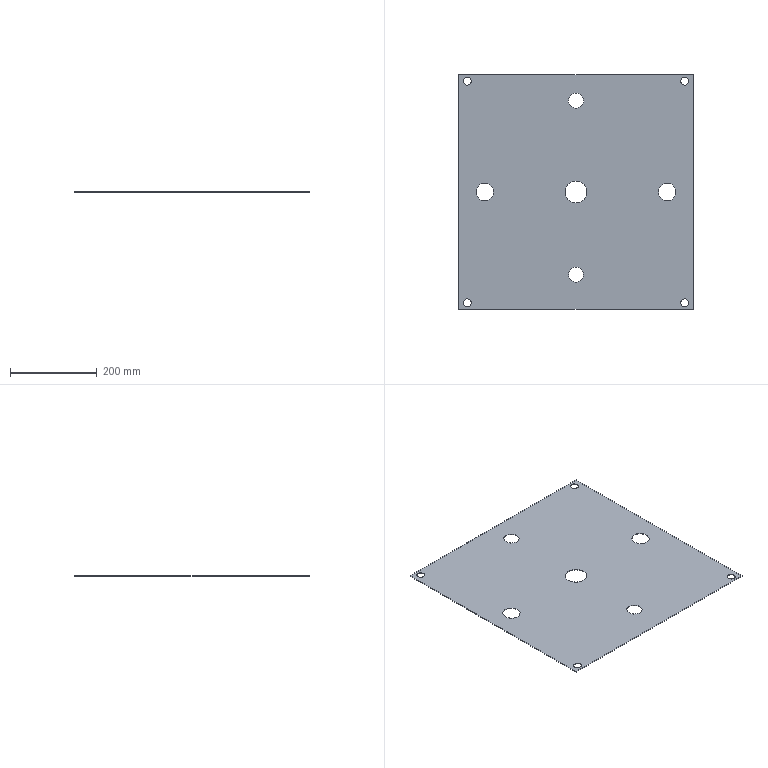Part | SolidWorks | features Cut 2, ICE 2, Extrusion 1 | 1 solid | 24 faces | box 540 x 540 x 1 mm | volume 284181 mm3 | cylinder 18 | plane 6 | commonest cylinder face diameters 18 x8 35 x4 40 x4 50 x2
STEP:
#1=CARTESIAN_POINT('',(17.5,210.,1.));
#2=VERTEX_POINT('',#1);
#3=CARTESIAN_POINT('',(-17.5,210.,1.));
#4=VERTEX_POINT('',#3);
#5=CARTESIAN_POINT('',(0.,210.,1.));
#6=DIRECTION('',(0.,0.,-1.));
#7=DIRECTION('',(-1.,0.,0.));
#8=AXIS2_PLACEMENT_3D('',#5,#6,#7);
#9=CIRCLE('',#8,17.5);
#10=EDGE_CURVE('',#2,#4,#9,.T.);
#11=ORIENTED_EDGE('',*,*,#10,.F.);
#12=CARTESIAN_POINT('',(17.5,210.,0.));
#13=VERTEX_POINT('',#12);
#14=CARTESIAN_POINT('',(17.5,210.,1.));
#15=DIRECTION('',(0.,0.,-1.));
#16=VECTOR('',#15,1000.);
#17=LINE('',#14,#16);
#18=EDGE_CURVE('',#2,#13,#17,.T.);
#19=ORIENTED_EDGE('',*,*,#18,.T.);
#20=CARTESIAN_POINT('',(-17.5,210.,0.));
#21=VERTEX_POINT('',#20);
#22=CARTESIAN_POINT('',(0.,210.,0.));
#23=DIRECTION('',(0.,0.,-1.));
#24=DIRECTION('',(-1.,0.,0.));
#25=AXIS2_PLACEMENT_3D('',#22,#23,#24);
#26=CIRCLE('',#25,17.5);
#27=EDGE_CURVE('',#13,#21,#26,.T.);
#28=ORIENTED_EDGE('',*,*,#27,.T.);
#29=CARTESIAN_POINT('',(-17.5,210.,1.));
#30=DIRECTION('',(0.,0.,-1.));
#31=VECTOR('',#30,1000.);
#32=LINE('',#29,#31);
#33=EDGE_CURVE('',#4,#21,#32,.T.);
#34=ORIENTED_EDGE('',*,*,#33,.F.);
#35=EDGE_LOOP('',(#11,#19,#28,#34));
#36=FACE_OUTER_BOUND('',#35,.T.);
#37=CARTESIAN_POINT('',(0.,210.,1.));
#38=DIRECTION('',(0.,0.,-1.));
#39=DIRECTION('',(-1.,0.,0.));
#40=AXIS2_PLACEMENT_3D('',#37,#38,#39);
#41=CYLINDRICAL_SURFACE('',#40,17.5);
#42=ADVANCED_FACE('',(#36),#41,.F.);
#43=CARTESIAN_POINT('',(17.5,-190.,1.));
#44=VERTEX_POINT('',#43);
#45=CARTESIAN_POINT('',(-17.5,-190.,1.));
#46=VERTEX_POINT('',#45);
#47=CARTESIAN_POINT('',(0.,-190.,1.));
#48=DIRECTION('',(0.,0.,-1.));
#49=DIRECTION('',(-1.,0.,0.));
#50=AXIS2_PLACEMENT_3D('',#47,#48,#49);
#51=CIRCLE('',#50,17.5);
#52=EDGE_CURVE('',#44,#46,#51,.T.);
#53=ORIENTED_EDGE('',*,*,#52,.F.);
#54=CARTESIAN_POINT('',(17.5,-190.,0.));
#55=VERTEX_POINT('',#54);
#56=CARTESIAN_POINT('',(17.5,-190.,1.));
#57=DIRECTION('',(0.,0.,-1.));
#58=VECTOR('',#57,1000.);
#59=LINE('',#56,#58);
#60=EDGE_CURVE('',#44,#55,#59,.T.);
#61=ORIENTED_EDGE('',*,*,#60,.T.);
#62=CARTESIAN_POINT('',(-17.5,-190.,0.));
#63=VERTEX_POINT('',#62);
#64=CARTESIAN_POINT('',(0.,-190.,0.));
#65=DIRECTION('',(0.,0.,-1.));
#66=DIRECTION('',(-1.,0.,0.));
#67=AXIS2_PLACEMENT_3D('',#64,#65,#66);
#68=CIRCLE('',#67,17.5);
#69=EDGE_CURVE('',#55,#63,#68,.T.);
#70=ORIENTED_EDGE('',*,*,#69,.T.);
#71=CARTESIAN_POINT('',(-17.5,-190.,1.));
#72=DIRECTION('',(0.,0.,-1.));
#73=VECTOR('',#72,1000.);
#74=LINE('',#71,#73);
#75=EDGE_CURVE('',#46,#63,#74,.T.);
#76=ORIENTED_EDGE('',*,*,#75,.F.);
#77=EDGE_LOOP('',(#53,#61,#70,#76));
#78=FACE_OUTER_BOUND('',#77,.T.);
#79=CARTESIAN_POINT('',(0.,-190.,1.));
#80=DIRECTION('',(0.,0.,-1.));
#81=DIRECTION('',(-1.,0.,0.));
#82=AXIS2_PLACEMENT_3D('',#79,#80,#81);
#83=CYLINDRICAL_SURFACE('',#82,17.5);
#84=ADVANCED_FACE('',(#78),#83,.F.);
#85=CARTESIAN_POINT('',(-25.,0.,0.));
#86=VERTEX_POINT('',#85);
#87=CARTESIAN_POINT('',(25.,0.,0.));
#88=VERTEX_POINT('',#87);
#89=CARTESIAN_POINT('',(0.,0.,0.));
#90=DIRECTION('',(0.,0.,1.));
#91=DIRECTION('',(1.,0.,0.));
#92=AXIS2_PLACEMENT_3D('',#89,#90,#91);
#93=CIRCLE('',#92,25.);
#94=EDGE_CURVE('',#86,#88,#93,.T.);
#95=ORIENTED_EDGE('',*,*,#94,.F.);
#96=CARTESIAN_POINT('',(-25.,0.,1.));
#97=VERTEX_POINT('',#96);
#98=CARTESIAN_POINT('',(-25.,0.,-9.));
#99=DIRECTION('',(0.,0.,1.));
#100=VECTOR('',#99,1000.);
#101=LINE('',#98,#100);
#102=EDGE_CURVE('',#86,#97,#101,.T.);
#103=ORIENTED_EDGE('',*,*,#102,.T.);
#104=CARTESIAN_POINT('',(25.,0.,1.));
#105=VERTEX_POINT('',#104);
#106=CARTESIAN_POINT('',(0.,0.,1.));
#107=DIRECTION('',(0.,0.,1.));
#108=DIRECTION('',(1.,0.,0.));
#109=AXIS2_PLACEMENT_3D('',#106,#107,#108);
#110=CIRCLE('',#109,25.);
#111=EDGE_CURVE('',#97,#105,#110,.T.);
#112=ORIENTED_EDGE('',*,*,#111,.T.);
#113=CARTESIAN_POINT('',(25.,0.,-9.));
#114=DIRECTION('',(0.,0.,1.));
#115=VECTOR('',#114,1000.);
#116=LINE('',#113,#115);
#117=EDGE_CURVE('',#88,#105,#116,.T.);
#118=ORIENTED_EDGE('',*,*,#117,.F.);
#119=EDGE_LOOP('',(#95,#103,#112,#118));
#120=FACE_OUTER_BOUND('',#119,.T.);
#121=CARTESIAN_POINT('',(0.,0.,-9.));
#122=DIRECTION('',(0.,0.,1.));
#123=DIRECTION('',(1.,0.,0.));
#124=AXIS2_PLACEMENT_3D('',#121,#122,#123);
#125=CYLINDRICAL_SURFACE('',#124,25.);
#126=ADVANCED_FACE('',(#120),#125,.F.);
#127=CARTESIAN_POINT('',(190.,0.,0.));
#128=VERTEX_POINT('',#127);
#129=CARTESIAN_POINT('',(230.,0.,0.));
#130=VERTEX_POINT('',#129);
#131=CARTESIAN_POINT('',(210.,0.,0.));
#132=DIRECTION('',(0.,0.,1.));
#133=DIRECTION('',(1.,0.,0.));
#134=AXIS2_PLACEMENT_3D('',#131,#132,#133);
#135=CIRCLE('',#134,20.);
#136=EDGE_CURVE('',#128,#130,#135,.T.);
#137=ORIENTED_EDGE('',*,*,#136,.F.);
#138=CARTESIAN_POINT('',(190.,0.,1.));
#139=VERTEX_POINT('',#138);
#140=CARTESIAN_POINT('',(190.,0.,0.));
#141=DIRECTION('',(0.,0.,1.));
#142=VECTOR('',#141,1000.);
#143=LINE('',#140,#142);
#144=EDGE_CURVE('',#128,#139,#143,.T.);
#145=ORIENTED_EDGE('',*,*,#144,.T.);
#146=CARTESIAN_POINT('',(230.,0.,1.));
#147=VERTEX_POINT('',#146);
#148=CARTESIAN_POINT('',(210.,0.,1.));
#149=DIRECTION('',(0.,0.,1.));
#150=DIRECTION('',(1.,0.,0.));
#151=AXIS2_PLACEMENT_3D('',#148,#149,#150);
#152=CIRCLE('',#151,20.);
#153=EDGE_CURVE('',#139,#147,#152,.T.);
#154=ORIENTED_EDGE('',*,*,#153,.T.);
#155=CARTESIAN_POINT('',(230.,0.,0.));
#156=DIRECTION('',(0.,0.,1.));
#157=VECTOR('',#156,1000.);
#158=LINE('',#155,#157);
#159=EDGE_CURVE('',#130,#147,#158,.T.);
#160=ORIENTED_EDGE('',*,*,#159,.F.);
#161=EDGE_LOOP('',(#137,#145,#154,#160));
#162=FACE_OUTER_BOUND('',#161,.T.);
#163=CARTESIAN_POINT('',(210.,0.,0.));
#164=DIRECTION('',(0.,0.,1.));
#165=DIRECTION('',(1.,0.,0.));
#166=AXIS2_PLACEMENT_3D('',#163,#164,#165);
#167=CYLINDRICAL_SURFACE('',#166,20.);
#168=ADVANCED_FACE('',(#162),#167,.F.);
#169=CARTESIAN_POINT('',(-230.,0.,0.));
#170=VERTEX_POINT('',#169);
#171=CARTESIAN_POINT('',(-190.,0.,0.));
#172=VERTEX_POINT('',#171);
#173=CARTESIAN_POINT('',(-210.,0.,0.));
#174=DIRECTION('',(0.,0.,1.));
#175=DIRECTION('',(1.,0.,0.));
#176=AXIS2_PLACEMENT_3D('',#173,#174,#175);
#177=CIRCLE('',#176,20.);
#178=EDGE_CURVE('',#170,#172,#177,.T.);
#179=ORIENTED_EDGE('',*,*,#178,.F.);
#180=CARTESIAN_POINT('',(-230.,0.,1.));
#181=VERTEX_POINT('',#180);
#182=CARTESIAN_POINT('',(-230.,0.,0.));
#183=DIRECTION('',(0.,0.,1.));
#184=VECTOR('',#183,1000.);
#185=LINE('',#182,#184);
#186=EDGE_CURVE('',#170,#181,#185,.T.);
#187=ORIENTED_EDGE('',*,*,#186,.T.);
#188=CARTESIAN_POINT('',(-190.,0.,1.));
#189=VERTEX_POINT('',#188);
#190=CARTESIAN_POINT('',(-210.,0.,1.));
#191=DIRECTION('',(0.,0.,1.));
#192=DIRECTION('',(1.,0.,0.));
#193=AXIS2_PLACEMENT_3D('',#190,#191,#192);
#194=CIRCLE('',#193,20.);
#195=EDGE_CURVE('',#181,#189,#194,.T.);
#196=ORIENTED_EDGE('',*,*,#195,.T.);
#197=CARTESIAN_POINT('',(-190.,0.,0.));
#198=DIRECTION('',(0.,0.,1.));
#199=VECTOR('',#198,1000.);
#200=LINE('',#197,#199);
#201=EDGE_CURVE('',#172,#189,#200,.T.);
#202=ORIENTED_EDGE('',*,*,#201,.F.);
#203=EDGE_LOOP('',(#179,#187,#196,#202));
#204=FACE_OUTER_BOUND('',#203,.T.);
#205=CARTESIAN_POINT('',(-210.,0.,0.));
#206=DIRECTION('',(0.,0.,1.));
#207=DIRECTION('',(1.,0.,0.));
#208=AXIS2_PLACEMENT_3D('',#205,#206,#207);
#209=CYLINDRICAL_SURFACE('',#208,20.);
#210=ADVANCED_FACE('',(#204),#209,.F.);
#211=CARTESIAN_POINT('',(259.,255.,1.));
#212=VERTEX_POINT('',#211);
#213=CARTESIAN_POINT('',(241.,255.,1.));
#214=VERTEX_POINT('',#213);
#215=CARTESIAN_POINT('',(250.,255.,1.));
#216=DIRECTION('',(0.,0.,-1.));
#217=DIRECTION('',(-1.,0.,0.));
#218=AXIS2_PLACEMENT_3D('',#215,#216,#217);
#219=CIRCLE('',#218,9.);
#220=EDGE_CURVE('',#212,#214,#219,.T.);
#221=ORIENTED_EDGE('',*,*,#220,.F.);
#222=CARTESIAN_POINT('',(259.,255.,0.));
#223=VERTEX_POINT('',#222);
#224=CARTESIAN_POINT('',(259.,255.,1.));
#225=DIRECTION('',(0.,0.,-1.));
#226=VECTOR('',#225,1000.);
#227=LINE('',#224,#226);
#228=EDGE_CURVE('',#212,#223,#227,.T.);
#229=ORIENTED_EDGE('',*,*,#228,.T.);
#230=CARTESIAN_POINT('',(241.,255.,0.));
#231=VERTEX_POINT('',#230);
#232=CARTESIAN_POINT('',(250.,255.,0.));
#233=DIRECTION('',(0.,0.,-1.));
#234=DIRECTION('',(-1.,0.,0.));
#235=AXIS2_PLACEMENT_3D('',#232,#233,#234);
#236=CIRCLE('',#235,9.);
#237=EDGE_CURVE('',#223,#231,#236,.T.);
#238=ORIENTED_EDGE('',*,*,#237,.T.);
#239=CARTESIAN_POINT('',(241.,255.,1.));
#240=DIRECTION('',(0.,0.,-1.));
#241=VECTOR('',#240,1000.);
#242=LINE('',#239,#241);
#243=EDGE_CURVE('',#214,#231,#242,.T.);
#244=ORIENTED_EDGE('',*,*,#243,.F.);
#245=EDGE_LOOP('',(#221,#229,#238,#244));
#246=FACE_OUTER_BOUND('',#245,.T.);
#247=CARTESIAN_POINT('',(250.,255.,1.));
#248=DIRECTION('',(0.,0.,-1.));
#249=DIRECTION('',(-1.,0.,0.));
#250=AXIS2_PLACEMENT_3D('',#247,#248,#249);
#251=CYLINDRICAL_SURFACE('',#250,9.);
#252=ADVANCED_FACE('',(#246),#251,.F.);
#253=CARTESIAN_POINT('',(-241.,255.,1.));
#254=VERTEX_POINT('',#253);
#255=CARTESIAN_POINT('',(-259.,255.,1.));
#256=VERTEX_POINT('',#255);
#257=CARTESIAN_POINT('',(-250.,255.,1.));
#258=DIRECTION('',(0.,0.,-1.));
#259=DIRECTION('',(-1.,0.,0.));
#260=AXIS2_PLACEMENT_3D('',#257,#258,#259);
#261=CIRCLE('',#260,9.);
#262=EDGE_CURVE('',#254,#256,#261,.T.);
#263=ORIENTED_EDGE('',*,*,#262,.F.);
#264=CARTESIAN_POINT('',(-241.,255.,0.));
#265=VERTEX_POINT('',#264);
#266=CARTESIAN_POINT('',(-241.,255.,1.));
#267=DIRECTION('',(0.,0.,-1.));
#268=VECTOR('',#267,1000.);
#269=LINE('',#266,#268);
#270=EDGE_CURVE('',#254,#265,#269,.T.);
#271=ORIENTED_EDGE('',*,*,#270,.T.);
#272=CARTESIAN_POINT('',(-259.,255.,0.));
#273=VERTEX_POINT('',#272);
#274=CARTESIAN_POINT('',(-250.,255.,0.));
#275=DIRECTION('',(0.,0.,-1.));
#276=DIRECTION('',(-1.,0.,0.));
#277=AXIS2_PLACEMENT_3D('',#274,#275,#276);
#278=CIRCLE('',#277,9.);
#279=EDGE_CURVE('',#265,#273,#278,.T.);
#280=ORIENTED_EDGE('',*,*,#279,.T.);
#281=CARTESIAN_POINT('',(-259.,255.,1.));
#282=DIRECTION('',(0.,0.,-1.));
#283=VECTOR('',#282,1000.);
#284=LINE('',#281,#283);
#285=EDGE_CURVE('',#256,#273,#284,.T.);
#286=ORIENTED_EDGE('',*,*,#285,.F.);
#287=EDGE_LOOP('',(#263,#271,#280,#286));
#288=FACE_OUTER_BOUND('',#287,.T.);
#289=CARTESIAN_POINT('',(-250.,255.,1.));
#290=DIRECTION('',(0.,0.,-1.));
#291=DIRECTION('',(-1.,0.,0.));
#292=AXIS2_PLACEMENT_3D('',#289,#290,#291);
#293=CYLINDRICAL_SURFACE('',#292,9.);
#294=ADVANCED_FACE('',(#288),#293,.F.);
#295=CARTESIAN_POINT('',(259.,-255.,1.));
#296=VERTEX_POINT('',#295);
#297=CARTESIAN_POINT('',(241.,-255.,1.));
#298=VERTEX_POINT('',#297);
#299=CARTESIAN_POINT('',(250.,-255.,1.));
#300=DIRECTION('',(0.,0.,-1.));
#301=DIRECTION('',(-1.,0.,0.));
#302=AXIS2_PLACEMENT_3D('',#299,#300,#301);
#303=CIRCLE('',#302,9.);
#304=EDGE_CURVE('',#296,#298,#303,.T.);
#305=ORIENTED_EDGE('',*,*,#304,.F.);
#306=CARTESIAN_POINT('',(259.,-255.,0.));
#307=VERTEX_POINT('',#306);
#308=CARTESIAN_POINT('',(259.,-255.,1.));
#309=DIRECTION('',(0.,0.,-1.));
#310=VECTOR('',#309,1000.);
#311=LINE('',#308,#310);
#312=EDGE_CURVE('',#296,#307,#311,.T.);
#313=ORIENTED_EDGE('',*,*,#312,.T.);
#314=CARTESIAN_POINT('',(241.,-255.,0.));
#315=VERTEX_POINT('',#314);
#316=CARTESIAN_POINT('',(250.,-255.,0.));
#317=DIRECTION('',(0.,0.,-1.));
#318=DIRECTION('',(-1.,0.,0.));
#319=AXIS2_PLACEMENT_3D('',#316,#317,#318);
#320=CIRCLE('',#319,9.);
#321=EDGE_CURVE('',#307,#315,#320,.T.);
#322=ORIENTED_EDGE('',*,*,#321,.T.);
#323=CARTESIAN_POINT('',(241.,-255.,1.));
#324=DIRECTION('',(0.,0.,-1.));
#325=VECTOR('',#324,1000.);
#326=LINE('',#323,#325);
#327=EDGE_CURVE('',#298,#315,#326,.T.);
#328=ORIENTED_EDGE('',*,*,#327,.F.);
#329=EDGE_LOOP('',(#305,#313,#322,#328));
#330=FACE_OUTER_BOUND('',#329,.T.);
#331=CARTESIAN_POINT('',(250.,-255.,1.));
#332=DIRECTION('',(0.,0.,-1.));
#333=DIRECTION('',(-1.,0.,0.));
#334=AXIS2_PLACEMENT_3D('',#331,#332,#333);
#335=CYLINDRICAL_SURFACE('',#334,9.);
#336=ADVANCED_FACE('',(#330),#335,.F.);
#337=CARTESIAN_POINT('',(-241.,-255.,1.));
#338=VERTEX_POINT('',#337);
#339=CARTESIAN_POINT('',(-259.,-255.,1.));
#340=VERTEX_POINT('',#339);
#341=CARTESIAN_POINT('',(-250.,-255.,1.));
#342=DIRECTION('',(0.,0.,-1.));
#343=DIRECTION('',(-1.,0.,0.));
#344=AXIS2_PLACEMENT_3D('',#341,#342,#343);
#345=CIRCLE('',#344,9.);
#346=EDGE_CURVE('',#338,#340,#345,.T.);
#347=ORIENTED_EDGE('',*,*,#346,.F.);
#348=CARTESIAN_POINT('',(-241.,-255.,0.));
#349=VERTEX_POINT('',#348);
#350=CARTESIAN_POINT('',(-241.,-255.,1.));
#351=DIRECTION('',(0.,0.,-1.));
#352=VECTOR('',#351,1000.);
#353=LINE('',#350,#352);
#354=EDGE_CURVE('',#338,#349,#353,.T.);
#355=ORIENTED_EDGE('',*,*,#354,.T.);
#356=CARTESIAN_POINT('',(-259.,-255.,0.));
#357=VERTEX_POINT('',#356);
#358=CARTESIAN_POINT('',(-250.,-255.,0.));
#359=DIRECTION('',(0.,0.,-1.));
#360=DIRECTION('',(-1.,0.,0.));
#361=AXIS2_PLACEMENT_3D('',#358,#359,#360);
#362=CIRCLE('',#361,9.);
#363=EDGE_CURVE('',#349,#357,#362,.T.);
#364=ORIENTED_EDGE('',*,*,#363,.T.);
#365=CARTESIAN_POINT('',(-259.,-255.,1.));
#366=DIRECTION('',(0.,0.,-1.));
#367=VECTOR('',#366,1000.);
#368=LINE('',#365,#367);
#369=EDGE_CURVE('',#340,#357,#368,.T.);
#370=ORIENTED_EDGE('',*,*,#369,.F.);
#371=EDGE_LOOP('',(#347,#355,#364,#370));
#372=FACE_OUTER_BOUND('',#371,.T.);
#373=CARTESIAN_POINT('',(-250.,-255.,1.));
#374=DIRECTION('',(0.,0.,-1.));
#375=DIRECTION('',(-1.,0.,0.));
#376=AXIS2_PLACEMENT_3D('',#373,#374,#375);
#377=CYLINDRICAL_SURFACE('',#376,9.);
#378=ADVANCED_FACE('',(#372),#377,.F.);
#379=CARTESIAN_POINT('',(270.,-270.,0.));
#380=VERTEX_POINT('',#379);
#381=CARTESIAN_POINT('',(270.,270.,0.));
#382=VERTEX_POINT('',#381);
#383=CARTESIAN_POINT('',(270.,270.,0.));
#384=DIRECTION('',(0.,1.,0.));
#385=VECTOR('',#384,1000.);
#386=LINE('',#383,#385);
#387=EDGE_CURVE('',#380,#382,#386,.T.);
#388=ORIENTED_EDGE('',*,*,#387,.T.);
#389=CARTESIAN_POINT('',(270.,270.,1.));
#390=VERTEX_POINT('',#389);
#391=CARTESIAN_POINT('',(270.,270.,1.));
#392=DIRECTION('',(0.,0.,-1.));
#393=VECTOR('',#392,1000.);
#394=LINE('',#391,#393);
#395=EDGE_CURVE('',#390,#382,#394,.T.);
#396=ORIENTED_EDGE('',*,*,#395,.F.);
#397=CARTESIAN_POINT('',(270.,-270.,1.));
#398=VERTEX_POINT('',#397);
#399=CARTESIAN_POINT('',(270.,270.,1.));
#400=DIRECTION('',(0.,1.,0.));
#401=VECTOR('',#400,1000.);
#402=LINE('',#399,#401);
#403=EDGE_CURVE('',#398,#390,#402,.T.);
#404=ORIENTED_EDGE('',*,*,#403,.F.);
#405=CARTESIAN_POINT('',(270.,-270.,1.));
#406=DIRECTION('',(0.,0.,-1.));
#407=VECTOR('',#406,1000.);
#408=LINE('',#405,#407);
#409=EDGE_CURVE('',#398,#380,#408,.T.);
#410=ORIENTED_EDGE('',*,*,#409,.T.);
#411=EDGE_LOOP('',(#388,#396,#404,#410));
#412=FACE_OUTER_BOUND('',#411,.T.);
#413=CARTESIAN_POINT('',(270.,270.,1.));
#414=DIRECTION('',(-1.,0.,0.));
#415=DIRECTION('',(0.,-1.,0.));
#416=AXIS2_PLACEMENT_3D('',#413,#414,#415);
#417=PLANE('',#416);
#418=ADVANCED_FACE('',(#412),#417,.F.);
#419=CARTESIAN_POINT('',(-270.,270.,0.));
#420=VERTEX_POINT('',#419);
#421=CARTESIAN_POINT('',(-270.,270.,0.));
#422=DIRECTION('',(-1.,0.,0.));
#423=VECTOR('',#422,1000.);
#424=LINE('',#421,#423);
#425=EDGE_CURVE('',#382,#420,#424,.T.);
#426=ORIENTED_EDGE('',*,*,#425,.T.);
#427=CARTESIAN_POINT('',(-270.,270.,1.));
#428=VERTEX_POINT('',#427);
#429=CARTESIAN_POINT('',(-270.,270.,1.));
#430=DIRECTION('',(0.,0.,-1.));
#431=VECTOR('',#430,1000.);
#432=LINE('',#429,#431);
#433=EDGE_CURVE('',#428,#420,#432,.T.);
#434=ORIENTED_EDGE('',*,*,#433,.F.);
#435=CARTESIAN_POINT('',(-270.,270.,1.));
#436=DIRECTION('',(-1.,0.,0.));
#437=VECTOR('',#436,1000.);
#438=LINE('',#435,#437);
#439=EDGE_CURVE('',#390,#428,#438,.T.);
#440=ORIENTED_EDGE('',*,*,#439,.F.);
#441=ORIENTED_EDGE('',*,*,#395,.T.);
#442=EDGE_LOOP('',(#426,#434,#440,#441));
#443=FACE_OUTER_BOUND('',#442,.T.);
#444=CARTESIAN_POINT('',(-270.,270.,1.));
#445=DIRECTION('',(0.,-1.,0.));
#446=DIRECTION('',(0.,0.,-1.));
#447=AXIS2_PLACEMENT_3D('',#444,#445,#446);
#448=PLANE('',#447);
#449=ADVANCED_FACE('',(#443),#448,.F.);
#450=CARTESIAN_POINT('',(-270.,-270.,0.));
#451=VERTEX_POINT('',#450);
#452=CARTESIAN_POINT('',(-270.,270.,0.));
#453=DIRECTION('',(0.,-1.,0.));
#454=VECTOR('',#453,1000.);
#455=LINE('',#452,#454);
#456=EDGE_CURVE('',#420,#451,#455,.T.);
#457=ORIENTED_EDGE('',*,*,#456,.T.);
#458=CARTESIAN_POINT('',(-270.,-270.,1.));
#459=VERTEX_POINT('',#458);
#460=CARTESIAN_POINT('',(-270.,-270.,1.));
#461=DIRECTION('',(0.,0.,-1.));
#462=VECTOR('',#461,1000.);
#463=LINE('',#460,#462);
#464=EDGE_CURVE('',#459,#451,#463,.T.);
#465=ORIENTED_EDGE('',*,*,#464,.F.);
#466=CARTESIAN_POINT('',(-270.,270.,1.));
#467=DIRECTION('',(0.,-1.,0.));
#468=VECTOR('',#467,1000.);
#469=LINE('',#466,#468);
#470=EDGE_CURVE('',#428,#459,#469,.T.);
#471=ORIENTED_EDGE('',*,*,#470,.F.);
#472=ORIENTED_EDGE('',*,*,#433,.T.);
#473=EDGE_LOOP('',(#457,#465,#471,#472));
#474=FACE_OUTER_BOUND('',#473,.T.);
#475=CARTESIAN_POINT('',(-270.,270.,1.));
#476=DIRECTION('',(1.,0.,0.));
#477=DIRECTION('',(0.,1.,0.));
#478=AXIS2_PLACEMENT_3D('',#475,#476,#477);
#479=PLANE('',#478);
#480=ADVANCED_FACE('',(#474),#479,.F.);
#481=CARTESIAN_POINT('',(-270.,-270.,0.));
#482=DIRECTION('',(1.,0.,0.));
#483=VECTOR('',#482,1000.);
#484=LINE('',#481,#483);
#485=EDGE_CURVE('',#451,#380,#484,.T.);
#486=ORIENTED_EDGE('',*,*,#485,.T.);
#487=ORIENTED_EDGE('',*,*,#409,.F.);
#488=CARTESIAN_POINT('',(-270.,-270.,1.));
#489=DIRECTION('',(1.,0.,0.));
#490=VECTOR('',#489,1000.);
#491=LINE('',#488,#490);
#492=EDGE_CURVE('',#459,#398,#491,.T.);
#493=ORIENTED_EDGE('',*,*,#492,.F.);
#494=ORIENTED_EDGE('',*,*,#464,.T.);
#495=EDGE_LOOP('',(#486,#487,#493,#494));
#496=FACE_OUTER_BOUND('',#495,.T.);
#497=CARTESIAN_POINT('',(-270.,-270.,1.));
#498=DIRECTION('',(0.,1.,0.));
#499=DIRECTION('',(0.,0.,1.));
#500=AXIS2_PLACEMENT_3D('',#497,#498,#499);
#501=PLANE('',#500);
#502=ADVANCED_FACE('',(#496),#501,.F.);
#503=CARTESIAN_POINT('',(0.,210.,1.));
#504=DIRECTION('',(0.,0.,-1.));
#505=DIRECTION('',(-1.,0.,0.));
#506=AXIS2_PLACEMENT_3D('',#503,#504,#505);
#507=CIRCLE('',#506,17.5);
#508=EDGE_CURVE('',#4,#2,#507,.T.);
#509=ORIENTED_EDGE('',*,*,#508,.T.);
#510=ORIENTED_EDGE('',*,*,#10,.T.);
#511=EDGE_LOOP('',(#509,#510));
#512=FACE_BOUND('',#511,.T.);
#513=CARTESIAN_POINT('',(0.,-190.,1.));
#514=DIRECTION('',(0.,0.,-1.));
#515=DIRECTION('',(-1.,0.,0.));
#516=AXIS2_PLACEMENT_3D('',#513,#514,#515);
#517=CIRCLE('',#516,17.5);
#518=EDGE_CURVE('',#46,#44,#517,.T.);
#519=ORIENTED_EDGE('',*,*,#518,.T.);
#520=ORIENTED_EDGE('',*,*,#52,.T.);
#521=EDGE_LOOP('',(#519,#520));
#522=FACE_BOUND('',#521,.T.);
#523=CARTESIAN_POINT('',(0.,0.,1.));
#524=DIRECTION('',(0.,0.,1.));
#525=DIRECTION('',(1.,0.,0.));
#526=AXIS2_PLACEMENT_3D('',#523,#524,#525);
#527=CIRCLE('',#526,25.);
#528=EDGE_CURVE('',#105,#97,#527,.T.);
#529=ORIENTED_EDGE('',*,*,#528,.F.);
#530=ORIENTED_EDGE('',*,*,#111,.F.);
#531=EDGE_LOOP('',(#529,#530));
#532=FACE_BOUND('',#531,.T.);
#533=CARTESIAN_POINT('',(210.,0.,1.));
#534=DIRECTION('',(0.,0.,1.));
#535=DIRECTION('',(1.,0.,0.));
#536=AXIS2_PLACEMENT_3D('',#533,#534,#535);
#537=CIRCLE('',#536,20.);
#538=EDGE_CURVE('',#147,#139,#537,.T.);
#539=ORIENTED_EDGE('',*,*,#538,.F.);
#540=ORIENTED_EDGE('',*,*,#153,.F.);
#541=EDGE_LOOP('',(#539,#540));
#542=FACE_BOUND('',#541,.T.);
#543=CARTESIAN_POINT('',(-210.,0.,1.));
#544=DIRECTION('',(0.,0.,1.));
#545=DIRECTION('',(1.,0.,0.));
#546=AXIS2_PLACEMENT_3D('',#543,#544,#545);
#547=CIRCLE('',#546,20.);
#548=EDGE_CURVE('',#189,#181,#547,.T.);
#549=ORIENTED_EDGE('',*,*,#548,.F.);
#550=ORIENTED_EDGE('',*,*,#195,.F.);
#551=EDGE_LOOP('',(#549,#550));
#552=FACE_BOUND('',#551,.T.);
#553=CARTESIAN_POINT('',(250.,255.,1.));
#554=DIRECTION('',(0.,0.,-1.));
#555=DIRECTION('',(-1.,0.,0.));
#556=AXIS2_PLACEMENT_3D('',#553,#554,#555);
#557=CIRCLE('',#556,9.);
#558=EDGE_CURVE('',#214,#212,#557,.T.);
#559=ORIENTED_EDGE('',*,*,#558,.T.);
#560=ORIENTED_EDGE('',*,*,#220,.T.);
#561=EDGE_LOOP('',(#559,#560));
#562=FACE_BOUND('',#561,.T.);
#563=CARTESIAN_POINT('',(-250.,255.,1.));
#564=DIRECTION('',(0.,0.,-1.));
#565=DIRECTION('',(-1.,0.,0.));
#566=AXIS2_PLACEMENT_3D('',#563,#564,#565);
#567=CIRCLE('',#566,9.);
#568=EDGE_CURVE('',#256,#254,#567,.T.);
#569=ORIENTED_EDGE('',*,*,#568,.T.);
#570=ORIENTED_EDGE('',*,*,#262,.T.);
#571=EDGE_LOOP('',(#569,#570));
#572=FACE_BOUND('',#571,.T.);
#573=CARTESIAN_POINT('',(250.,-255.,1.));
#574=DIRECTION('',(0.,0.,-1.));
#575=DIRECTION('',(-1.,0.,0.));
#576=AXIS2_PLACEMENT_3D('',#573,#574,#575);
#577=CIRCLE('',#576,9.);
#578=EDGE_CURVE('',#298,#296,#577,.T.);
#579=ORIENTED_EDGE('',*,*,#578,.T.);
#580=ORIENTED_EDGE('',*,*,#304,.T.);
#581=EDGE_LOOP('',(#579,#580));
#582=FACE_BOUND('',#581,.T.);
#583=CARTESIAN_POINT('',(-250.,-255.,1.));
#584=DIRECTION('',(0.,0.,-1.));
#585=DIRECTION('',(-1.,0.,0.));
#586=AXIS2_PLACEMENT_3D('',#583,#584,#585);
#587=CIRCLE('',#586,9.);
#588=EDGE_CURVE('',#340,#338,#587,.T.);
#589=ORIENTED_EDGE('',*,*,#588,.T.);
#590=ORIENTED_EDGE('',*,*,#346,.T.);
#591=EDGE_LOOP('',(#589,#590));
#592=FACE_BOUND('',#591,.T.);
#593=ORIENTED_EDGE('',*,*,#403,.T.);
#594=ORIENTED_EDGE('',*,*,#439,.T.);
#595=ORIENTED_EDGE('',*,*,#470,.T.);
#596=ORIENTED_EDGE('',*,*,#492,.T.);
#597=EDGE_LOOP('',(#593,#594,#595,#596));
#598=FACE_OUTER_BOUND('',#597,.T.);
#599=CARTESIAN_POINT('',(0.,0.,1.));
#600=DIRECTION('',(0.,0.,1.));
#601=DIRECTION('',(1.,0.,0.));
#602=AXIS2_PLACEMENT_3D('',#599,#600,#601);
#603=PLANE('',#602);
#604=ADVANCED_FACE('',(#512,#522,#532,#542,#552,#562,#572,#582,#592,#598),#603,.T.);
#605=CARTESIAN_POINT('',(0.,210.,0.));
#606=DIRECTION('',(0.,0.,-1.));
#607=DIRECTION('',(-1.,0.,0.));
#608=AXIS2_PLACEMENT_3D('',#605,#606,#607);
#609=CIRCLE('',#608,17.5);
#610=EDGE_CURVE('',#21,#13,#609,.T.);
#611=ORIENTED_EDGE('',*,*,#610,.F.);
#612=ORIENTED_EDGE('',*,*,#27,.F.);
#613=EDGE_LOOP('',(#611,#612));
#614=FACE_BOUND('',#613,.T.);
#615=CARTESIAN_POINT('',(0.,-190.,0.));
#616=DIRECTION('',(0.,0.,-1.));
#617=DIRECTION('',(-1.,0.,0.));
#618=AXIS2_PLACEMENT_3D('',#615,#616,#617);
#619=CIRCLE('',#618,17.5);
#620=EDGE_CURVE('',#63,#55,#619,.T.);
#621=ORIENTED_EDGE('',*,*,#620,.F.);
#622=ORIENTED_EDGE('',*,*,#69,.F.);
#623=EDGE_LOOP('',(#621,#622));
#624=FACE_BOUND('',#623,.T.);
#625=CARTESIAN_POINT('',(0.,0.,0.));
#626=DIRECTION('',(0.,0.,1.));
#627=DIRECTION('',(1.,0.,0.));
#628=AXIS2_PLACEMENT_3D('',#625,#626,#627);
#629=CIRCLE('',#628,25.);
#630=EDGE_CURVE('',#88,#86,#629,.T.);
#631=ORIENTED_EDGE('',*,*,#630,.T.);
#632=ORIENTED_EDGE('',*,*,#94,.T.);
#633=EDGE_LOOP('',(#631,#632));
#634=FACE_BOUND('',#633,.T.);
#635=CARTESIAN_POINT('',(210.,0.,0.));
#636=DIRECTION('',(0.,0.,1.));
#637=DIRECTION('',(1.,0.,0.));
#638=AXIS2_PLACEMENT_3D('',#635,#636,#637);
#639=CIRCLE('',#638,20.);
#640=EDGE_CURVE('',#130,#128,#639,.T.);
#641=ORIENTED_EDGE('',*,*,#640,.T.);
#642=ORIENTED_EDGE('',*,*,#136,.T.);
#643=EDGE_LOOP('',(#641,#642));
#644=FACE_BOUND('',#643,.T.);
#645=CARTESIAN_POINT('',(-210.,0.,0.));
#646=DIRECTION('',(0.,0.,1.));
#647=DIRECTION('',(1.,0.,0.));
#648=AXIS2_PLACEMENT_3D('',#645,#646,#647);
#649=CIRCLE('',#648,20.);
#650=EDGE_CURVE('',#172,#170,#649,.T.);
#651=ORIENTED_EDGE('',*,*,#650,.T.);
#652=ORIENTED_EDGE('',*,*,#178,.T.);
#653=EDGE_LOOP('',(#651,#652));
#654=FACE_BOUND('',#653,.T.);
#655=CARTESIAN_POINT('',(250.,255.,0.));
#656=DIRECTION('',(0.,0.,-1.));
#657=DIRECTION('',(-1.,0.,0.));
#658=AXIS2_PLACEMENT_3D('',#655,#656,#657);
#659=CIRCLE('',#658,9.);
#660=EDGE_CURVE('',#231,#223,#659,.T.);
#661=ORIENTED_EDGE('',*,*,#660,.F.);
#662=ORIENTED_EDGE('',*,*,#237,.F.);
#663=EDGE_LOOP('',(#661,#662));
#664=FACE_BOUND('',#663,.T.);
#665=CARTESIAN_POINT('',(-250.,255.,0.));
#666=DIRECTION('',(0.,0.,-1.));
#667=DIRECTION('',(-1.,0.,0.));
#668=AXIS2_PLACEMENT_3D('',#665,#666,#667);
#669=CIRCLE('',#668,9.);
#670=EDGE_CURVE('',#273,#265,#669,.T.);
#671=ORIENTED_EDGE('',*,*,#670,.F.);
#672=ORIENTED_EDGE('',*,*,#279,.F.);
#673=EDGE_LOOP('',(#671,#672));
#674=FACE_BOUND('',#673,.T.);
#675=CARTESIAN_POINT('',(250.,-255.,0.));
#676=DIRECTION('',(0.,0.,-1.));
#677=DIRECTION('',(-1.,0.,0.));
#678=AXIS2_PLACEMENT_3D('',#675,#676,#677);
#679=CIRCLE('',#678,9.);
#680=EDGE_CURVE('',#315,#307,#679,.T.);
#681=ORIENTED_EDGE('',*,*,#680,.F.);
#682=ORIENTED_EDGE('',*,*,#321,.F.);
#683=EDGE_LOOP('',(#681,#682));
#684=FACE_BOUND('',#683,.T.);
#685=CARTESIAN_POINT('',(-250.,-255.,0.));
#686=DIRECTION('',(0.,0.,-1.));
#687=DIRECTION('',(-1.,0.,0.));
#688=AXIS2_PLACEMENT_3D('',#685,#686,#687);
#689=CIRCLE('',#688,9.);
#690=EDGE_CURVE('',#357,#349,#689,.T.);
#691=ORIENTED_EDGE('',*,*,#690,.F.);
#692=ORIENTED_EDGE('',*,*,#363,.F.);
#693=EDGE_LOOP('',(#691,#692));
#694=FACE_BOUND('',#693,.T.);
#695=ORIENTED_EDGE('',*,*,#387,.F.);
#696=ORIENTED_EDGE('',*,*,#485,.F.);
#697=ORIENTED_EDGE('',*,*,#456,.F.);
#698=ORIENTED_EDGE('',*,*,#425,.F.);
#699=EDGE_LOOP('',(#695,#696,#697,#698));
#700=FACE_OUTER_BOUND('',#699,.T.);
#701=CARTESIAN_POINT('',(0.,0.,0.));
#702=DIRECTION('',(0.,0.,1.));
#703=DIRECTION('',(1.,0.,0.));
#704=AXIS2_PLACEMENT_3D('',#701,#702,#703);
#705=PLANE('',#704);
#706=ADVANCED_FACE('',(#614,#624,#634,#644,#654,#664,#674,#684,#694,#700),#705,.F.);
#707=ORIENTED_EDGE('',*,*,#354,.F.);
#708=ORIENTED_EDGE('',*,*,#588,.F.);
#709=ORIENTED_EDGE('',*,*,#369,.T.);
#710=ORIENTED_EDGE('',*,*,#690,.T.);
#711=EDGE_LOOP('',(#707,#708,#709,#710));
#712=FACE_OUTER_BOUND('',#711,.T.);
#713=CARTESIAN_POINT('',(-250.,-255.,1.));
#714=DIRECTION('',(0.,0.,-1.));
#715=DIRECTION('',(-1.,0.,0.));
#716=AXIS2_PLACEMENT_3D('',#713,#714,#715);
#717=CYLINDRICAL_SURFACE('',#716,9.);
#718=ADVANCED_FACE('',(#712),#717,.F.);
#719=ORIENTED_EDGE('',*,*,#312,.F.);
#720=ORIENTED_EDGE('',*,*,#578,.F.);
#721=ORIENTED_EDGE('',*,*,#327,.T.);
#722=ORIENTED_EDGE('',*,*,#680,.T.);
#723=EDGE_LOOP('',(#719,#720,#721,#722));
#724=FACE_OUTER_BOUND('',#723,.T.);
#725=CARTESIAN_POINT('',(250.,-255.,1.));
#726=DIRECTION('',(0.,0.,-1.));
#727=DIRECTION('',(-1.,0.,0.));
#728=AXIS2_PLACEMENT_3D('',#725,#726,#727);
#729=CYLINDRICAL_SURFACE('',#728,9.);
#730=ADVANCED_FACE('',(#724),#729,.F.);
#731=ORIENTED_EDGE('',*,*,#270,.F.);
#732=ORIENTED_EDGE('',*,*,#568,.F.);
#733=ORIENTED_EDGE('',*,*,#285,.T.);
#734=ORIENTED_EDGE('',*,*,#670,.T.);
#735=EDGE_LOOP('',(#731,#732,#733,#734));
#736=FACE_OUTER_BOUND('',#735,.T.);
#737=CARTESIAN_POINT('',(-250.,255.,1.));
#738=DIRECTION('',(0.,0.,-1.));
#739=DIRECTION('',(-1.,0.,0.));
#740=AXIS2_PLACEMENT_3D('',#737,#738,#739);
#741=CYLINDRICAL_SURFACE('',#740,9.);
#742=ADVANCED_FACE('',(#736),#741,.F.);
#743=ORIENTED_EDGE('',*,*,#228,.F.);
#744=ORIENTED_EDGE('',*,*,#558,.F.);
#745=ORIENTED_EDGE('',*,*,#243,.T.);
#746=ORIENTED_EDGE('',*,*,#660,.T.);
#747=EDGE_LOOP('',(#743,#744,#745,#746));
#748=FACE_OUTER_BOUND('',#747,.T.);
#749=CARTESIAN_POINT('',(250.,255.,1.));
#750=DIRECTION('',(0.,0.,-1.));
#751=DIRECTION('',(-1.,0.,0.));
#752=AXIS2_PLACEMENT_3D('',#749,#750,#751);
#753=CYLINDRICAL_SURFACE('',#752,9.);
#754=ADVANCED_FACE('',(#748),#753,.F.);
#755=ORIENTED_EDGE('',*,*,#186,.F.);
#756=ORIENTED_EDGE('',*,*,#650,.F.);
#757=ORIENTED_EDGE('',*,*,#201,.T.);
#758=ORIENTED_EDGE('',*,*,#548,.T.);
#759=EDGE_LOOP('',(#755,#756,#757,#758));
#760=FACE_OUTER_BOUND('',#759,.T.);
#761=CARTESIAN_POINT('',(-210.,0.,0.));
#762=DIRECTION('',(0.,0.,1.));
#763=DIRECTION('',(1.,0.,0.));
#764=AXIS2_PLACEMENT_3D('',#761,#762,#763);
#765=CYLINDRICAL_SURFACE('',#764,20.);
#766=ADVANCED_FACE('',(#760),#765,.F.);
#767=ORIENTED_EDGE('',*,*,#144,.F.);
#768=ORIENTED_EDGE('',*,*,#640,.F.);
#769=ORIENTED_EDGE('',*,*,#159,.T.);
#770=ORIENTED_EDGE('',*,*,#538,.T.);
#771=EDGE_LOOP('',(#767,#768,#769,#770));
#772=FACE_OUTER_BOUND('',#771,.T.);
#773=CARTESIAN_POINT('',(210.,0.,0.));
#774=DIRECTION('',(0.,0.,1.));
#775=DIRECTION('',(1.,0.,0.));
#776=AXIS2_PLACEMENT_3D('',#773,#774,#775);
#777=CYLINDRICAL_SURFACE('',#776,20.);
#778=ADVANCED_FACE('',(#772),#777,.F.);
#779=ORIENTED_EDGE('',*,*,#102,.F.);
#780=ORIENTED_EDGE('',*,*,#630,.F.);
#781=ORIENTED_EDGE('',*,*,#117,.T.);
#782=ORIENTED_EDGE('',*,*,#528,.T.);
#783=EDGE_LOOP('',(#779,#780,#781,#782));
#784=FACE_OUTER_BOUND('',#783,.T.);
#785=CARTESIAN_POINT('',(0.,0.,-9.));
#786=DIRECTION('',(0.,0.,1.));
#787=DIRECTION('',(1.,0.,0.));
#788=AXIS2_PLACEMENT_3D('',#785,#786,#787);
#789=CYLINDRICAL_SURFACE('',#788,25.);
#790=ADVANCED_FACE('',(#784),#789,.F.);
#791=ORIENTED_EDGE('',*,*,#60,.F.);
#792=ORIENTED_EDGE('',*,*,#518,.F.);
#793=ORIENTED_EDGE('',*,*,#75,.T.);
#794=ORIENTED_EDGE('',*,*,#620,.T.);
#795=EDGE_LOOP('',(#791,#792,#793,#794));
#796=FACE_OUTER_BOUND('',#795,.T.);
#797=CARTESIAN_POINT('',(0.,-190.,1.));
#798=DIRECTION('',(0.,0.,-1.));
#799=DIRECTION('',(-1.,0.,0.));
#800=AXIS2_PLACEMENT_3D('',#797,#798,#799);
#801=CYLINDRICAL_SURFACE('',#800,17.5);
#802=ADVANCED_FACE('',(#796),#801,.F.);
#803=ORIENTED_EDGE('',*,*,#18,.F.);
#804=ORIENTED_EDGE('',*,*,#508,.F.);
#805=ORIENTED_EDGE('',*,*,#33,.T.);
#806=ORIENTED_EDGE('',*,*,#610,.T.);
#807=EDGE_LOOP('',(#803,#804,#805,#806));
#808=FACE_OUTER_BOUND('',#807,.T.);
#809=CARTESIAN_POINT('',(0.,210.,1.));
#810=DIRECTION('',(0.,0.,-1.));
#811=DIRECTION('',(-1.,0.,0.));
#812=AXIS2_PLACEMENT_3D('',#809,#810,#811);
#813=CYLINDRICAL_SURFACE('',#812,17.5);
#814=ADVANCED_FACE('',(#808),#813,.F.);
#815=CLOSED_SHELL('',(#42,#84,#126,#168,#210,#252,#294,#336,#378,#418,#449,#480,#502,#604,#706,#718,#730,#742,#754,#766,#778,#790,#802,#814));
#816=MANIFOLD_SOLID_BREP('',#815);
#817=CARTESIAN_POINT('',(0.,0.,0.));
#818=DIRECTION('',(0.,0.,1.));
#819=DIRECTION('',(1.,0.,0.));
#820=AXIS2_PLACEMENT_3D('',#817,#818,#819);
#821=(LENGTH_UNIT()NAMED_UNIT(*)SI_UNIT(.MILLI.,.METRE.));
#822=UNCERTAINTY_MEASURE_WITH_UNIT(LENGTH_MEASURE(0.00001),#821,'','');
#823=(NAMED_UNIT(*)PLANE_ANGLE_UNIT()SI_UNIT($,.RADIAN.));
#824=(NAMED_UNIT(*)SI_UNIT($,.STERADIAN.)SOLID_ANGLE_UNIT());
#825=(GEOMETRIC_REPRESENTATION_CONTEXT(3)GLOBAL_UNCERTAINTY_ASSIGNED_CONTEXT((#822))GLOBAL_UNIT_ASSIGNED_CONTEXT((#821,#823,#824))REPRESENTATION_CONTEXT('',''));
#826=ADVANCED_BREP_SHAPE_REPRESENTATION('',(#816,#820),#825);